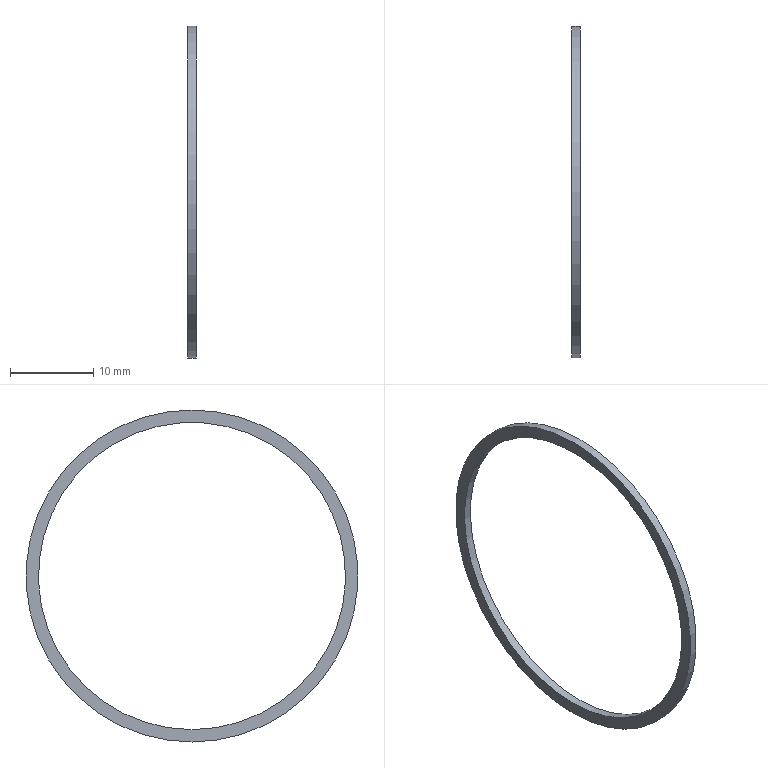Part | STEP file | Inner seal of clamping device 2 | 1 solid | 4 faces | box 1 x 40 x 40 mm | volume 181.427 mm3 | plane 2 | cylinder 2 | commonest cylinder face diameters 37 x1 40 x1
STEP:
#1=CARTESIAN_POINT('',(0.,0.,-20.));
#2=VERTEX_POINT('',#1);
#3=CARTESIAN_POINT('',(0.,0.,0.));
#4=DIRECTION('',(1.,0.,0.));
#5=DIRECTION('',(0.,0.,-1.));
#6=AXIS2_PLACEMENT_3D('',#3,#4,#5);
#7=CIRCLE('',#6,20.);
#8=EDGE_CURVE('',#2,#2,#7,.T.);
#9=ORIENTED_EDGE('',*,*,#8,.F.);
#10=EDGE_LOOP('',(#9));
#11=FACE_BOUND('',#10,.T.);
#12=CARTESIAN_POINT('',(0.,0.,-18.5));
#13=VERTEX_POINT('',#12);
#14=CARTESIAN_POINT('',(0.,0.,0.));
#15=DIRECTION('',(1.,0.,0.));
#16=DIRECTION('',(0.,0.,-1.));
#17=AXIS2_PLACEMENT_3D('',#14,#15,#16);
#18=CIRCLE('',#17,18.5);
#19=EDGE_CURVE('',#13,#13,#18,.T.);
#20=ORIENTED_EDGE('',*,*,#19,.T.);
#21=EDGE_LOOP('',(#20));
#22=FACE_BOUND('',#21,.T.);
#23=CARTESIAN_POINT('',(0.,0.,0.));
#24=DIRECTION('',(1.,0.,0.));
#25=DIRECTION('',(0.,0.,-1.));
#26=AXIS2_PLACEMENT_3D('',#23,#24,#25);
#27=PLANE('',#26);
#28=ADVANCED_FACE('',(#11,#22),#27,.F.);
#29=CARTESIAN_POINT('',(1.,0.,-20.));
#30=VERTEX_POINT('',#29);
#31=CARTESIAN_POINT('',(1.,0.,0.));
#32=DIRECTION('',(1.,0.,0.));
#33=DIRECTION('',(0.,0.,-1.));
#34=AXIS2_PLACEMENT_3D('',#31,#32,#33);
#35=CIRCLE('',#34,20.);
#36=EDGE_CURVE('',#30,#30,#35,.T.);
#37=ORIENTED_EDGE('',*,*,#36,.T.);
#38=EDGE_LOOP('',(#37));
#39=FACE_BOUND('',#38,.T.);
#40=CARTESIAN_POINT('',(1.,0.,-18.5));
#41=VERTEX_POINT('',#40);
#42=CARTESIAN_POINT('',(1.,0.,0.));
#43=DIRECTION('',(1.,0.,0.));
#44=DIRECTION('',(0.,0.,-1.));
#45=AXIS2_PLACEMENT_3D('',#42,#43,#44);
#46=CIRCLE('',#45,18.5);
#47=EDGE_CURVE('',#41,#41,#46,.F.);
#48=ORIENTED_EDGE('',*,*,#47,.T.);
#49=EDGE_LOOP('',(#48));
#50=FACE_BOUND('',#49,.T.);
#51=CARTESIAN_POINT('',(1.,0.,0.));
#52=DIRECTION('',(1.,0.,0.));
#53=DIRECTION('',(0.,0.,-1.));
#54=AXIS2_PLACEMENT_3D('',#51,#52,#53);
#55=PLANE('',#54);
#56=ADVANCED_FACE('',(#39,#50),#55,.T.);
#57=ORIENTED_EDGE('',*,*,#47,.F.);
#58=EDGE_LOOP('',(#57));
#59=FACE_OUTER_BOUND('',#58,.T.);
#60=ORIENTED_EDGE('',*,*,#19,.F.);
#61=EDGE_LOOP('',(#60));
#62=FACE_OUTER_BOUND('',#61,.T.);
#63=CARTESIAN_POINT('',(0.,0.,0.));
#64=DIRECTION('',(1.,0.,0.));
#65=DIRECTION('',(0.,0.,-1.));
#66=AXIS2_PLACEMENT_3D('',#63,#64,#65);
#67=CYLINDRICAL_SURFACE('',#66,18.5);
#68=ADVANCED_FACE('',(#59,#62),#67,.F.);
#69=ORIENTED_EDGE('',*,*,#36,.F.);
#70=EDGE_LOOP('',(#69));
#71=FACE_OUTER_BOUND('',#70,.T.);
#72=ORIENTED_EDGE('',*,*,#8,.T.);
#73=EDGE_LOOP('',(#72));
#74=FACE_OUTER_BOUND('',#73,.T.);
#75=CARTESIAN_POINT('',(0.,0.,0.));
#76=DIRECTION('',(1.,0.,0.));
#77=DIRECTION('',(0.,0.,-1.));
#78=AXIS2_PLACEMENT_3D('',#75,#76,#77);
#79=CYLINDRICAL_SURFACE('',#78,20.);
#80=ADVANCED_FACE('',(#71,#74),#79,.T.);
#81=CLOSED_SHELL('',(#28,#56,#68,#80));
#82=MANIFOLD_SOLID_BREP('',#81);
#83=(LENGTH_UNIT()NAMED_UNIT(*)SI_UNIT(.MILLI.,.METRE.));
#84=UNCERTAINTY_MEASURE_WITH_UNIT(LENGTH_MEASURE(0.00001),#83,'','');
#85=(NAMED_UNIT(*)PLANE_ANGLE_UNIT()SI_UNIT($,.RADIAN.));
#86=(NAMED_UNIT(*)SI_UNIT($,.STERADIAN.)SOLID_ANGLE_UNIT());
#87=(GEOMETRIC_REPRESENTATION_CONTEXT(3)GLOBAL_UNCERTAINTY_ASSIGNED_CONTEXT((#84))GLOBAL_UNIT_ASSIGNED_CONTEXT((#83,#85,#86))REPRESENTATION_CONTEXT('',''));
#88=ADVANCED_BREP_SHAPE_REPRESENTATION('',(#82),#87);